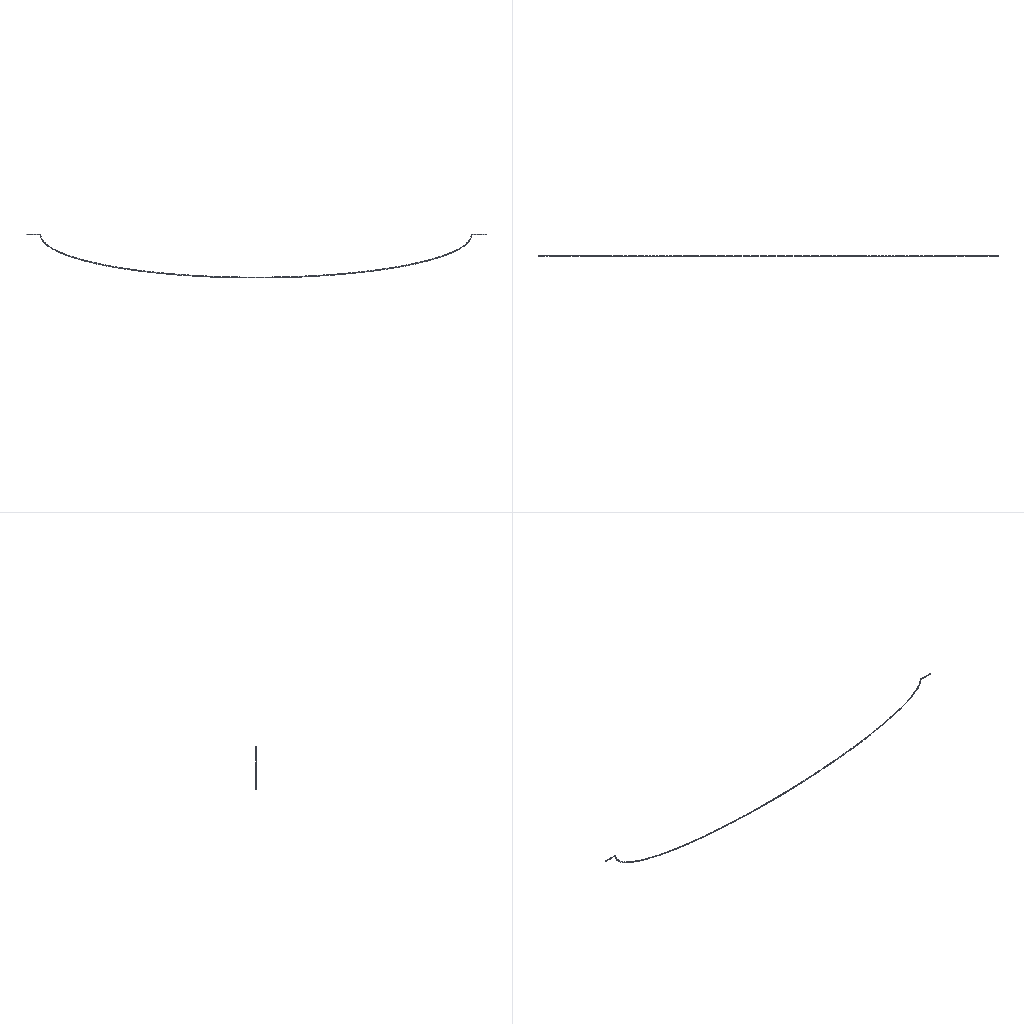Simulation study | ansys workbench
Set-up summary:
category,name,step,type,value,unit,region
solver,ansys_workbench
units,mm-N-s-tonne (MPa),,stated,"/units,MPA"
analysis,LS1,,modal,method=lanb; n_modes=6
load_step,LS1,LS1,modal
mesh,nodes,,,2790
mesh,elements,,,1023
element_type,SOLID187,,,1023
material,Structural Steel,,E,200000,tonne s^-2 mm^-1
material,Structural Steel,,nu,0.3
material,Structural Steel,,density,7.85e-09,tonne mm^-3
material,Structural Steel,,conductivity,60.5,tonne mm s^-3 C^-1
material,Structural Steel,,specific_heat,4.34e+08,mm^2 s^-2 C^-1
material,Structural Steel,,cte,1.2e-05,C^-1
material,Structural Steel,,permeability,10000
material,Structural Steel,,resistivity,0.00017,ohm mm
Ansys APDL input file, long lists of numbers shortened:
/batch
/config,noeldb,1     ! force off writing results to database
*get,_wallstrt,active,,time,wall
! ANSYS input file written by Workbench version 2022 R1
! File used for geometry attach:
/title,wbnew--__ (B5)
! ****** Begin Custom Load Command Snippet ******
/COM, ACT Extensions:
/COM,     LSDYNA, 2021.1
/COM,
! ****** End   Custom Load Command Snippet ******
*DIM,_wb_ProjectScratch_dir,string,248
_wb_ProjectScratch_dir(1) = ''
*DIM,_wb_SolverFiles_dir,string,248
_wb_SolverFiles_dir(1) = ''
*DIM,_wb_userfiles_dir,string,248
_wb_userfiles_dir(1) = ''
/com,--- Data in consistent NMM units. See Solving Units in the help system for more information.
/units,MPA
/nopr
/wb,file,start              !  signify a WB generated input file
/prep7
! Turn off shape checking because checks already performed inside WB mesher.
! See help system for more information.
SHPP,OFF,,NOWARN
/nolist
etcon,set             ! allow ANSYS to choose best KEYOP's for 180x elements, resets any applicable keyopt to MAPDL defaults
/com,*********** Nodes for the whole assembly ***********
nblock,3,,3069
(1i9,3e20.9e3)
        1     1.600000000E+04     0.000000000E+00     3.000000000E+01
! (2789 more lines like these left out)
-1
/wb,elem,start            !  set before creation of elements
/com,*********** Elements for Body 1 "__1-FreeParts|__1" ***********
et,1,187
eblock,19,solid,,1023
(19i9)
        1        1        1        1        0        0        0        0       10        0        1        2      151      589        4      599     1655      600      597
! (2045 more lines like these left out)
-1
/wb,elem,end               !  done creating elements
/com,*********** Send User Defined Coordinate System(s) ***********
csys,0
toffst,273.15,  ! Temperature offset from absolute zero
/com,*********** Set Reference Temperature ***********
tref,22.
/wb,mat,start              !  starting to send materials
/com,*********** Send Materials ***********
Temperature = 'TEMP' ! Temperature
MP,DENS,1,7.85e-09,	! tonne mm^-3
MP,ALPX,1,1.2e-05,	! C^-1
MP,C,1,434000000,	! mm^2 s^-2 C^-1
MP,KXX,1,60.5,	! tonne mm s^-3 C^-1
MP,RSVX,1,0.00017,	! ohm mm
MP,EX,1,200000,	! tonne s^-2 mm^-1
MP,NUXY,1,0.3,
MP,MURX,1,10000,
/wb,mat,end                !  done sending materials
!************************* Model Summary ********************
!__1-FreeParts|__1,	结构钢,	matid,	1
!************************* End Model Summary ********************
! get the diagonal of the bounding box. Needed later for other things
*get,_xmin,node,,mnloc,x
*get,_ymin,node,,mnloc,y
*get,_zmin,node,,mnloc,z
*get,_xmax,node,,mxloc,x
*get,_ymax,node,,mxloc,y
*get,_zmax,node,,mxloc,z
_ASMDIAG=(_xmax-_xmin)*(_xmax-_xmin)+(_ymax-_ymin)*(_ymax-_ymin)+(_zmax-_zmin)*(_zmax-_zmin)
_ASMDIAG=SQRT(_ASMDIAG)
/wb,contact,start          !  starting to send contact
/wb,contact,end            !  done creating contacts
/golist
/wb,load,start             !  starting to send loads
/gst,on,on
fini
*get,_numnode,node,0,count
*get,_numelem,elem,0,count
*get, _MAXELEMNUM, elem, 0, NUM, MAX
*get, _MAXNODENUM, node, 0, NUM, MAX
*get, _MAXELEMTYPE, etyp, 0, NUM, MAX
*get, _MAXREALCONST, real, 0, NUM, MAX
/go
/wb,load,end               !  done creating loads
/com,--- Number of total nodes = %_numnode%
/com,--- Number of contact elements = 0
/com,--- Number of spring elements = 0
/com,--- Number of bearing elements = 0
/com,--- Number of solid elements = 1023
/com,--- Number of condensed parts = 0
/com,--- Number of total elements = %_numelem%
*get,_wallbsol,active,,time,wall
/solu
antype,2                   ! modal analysis
_thickRatio=  0     ! Ratio of thick parts in the model
modopt,lanb,6
outres,erase
outres,all,none
outres,nsol,all
outres,etmp,all
mxpand                    ! default expand in case of complex solution
dmpopt,esav,no
dmpopt,emat,no
dmpopt,full,no
! *********** WB SOLVE COMMAND ***********
! check interactive state
*get,ANSINTER_,active,,int
*if,ANSINTER_,ne,0,then
/eof
*endif
solve
/com *************** Write FE CONNECTORS *********
CEWRITE,file,ce,,INTE
*get,_nmodalsolproc,active,0,numcpu
fini
/nopr
*get,_numnode,node,0,count
*get,_numelem,elem,0,count
*get, _MAXELEMNUM, elem, 0, NUM, MAX
*get, _MAXNODENUM, node, 0, NUM, MAX,,,INTERNAL
*get, _MAXELEMTYPE, etyp, 0, NUM, MAX
*get, _MAXREALCONST, real, 0, NUM, MAX
/gopr
*get,_wallasol,active,,time,wall
/post1
/nopr
*dim,_direction,CHAR,6,1
_direction(1) = 'X'
_direction(2) = 'Y'
_direction(3) = 'Z'
_direction(4) = 'ROTX'
_direction(5) = 'ROTY'
_direction(6) = 'ROTZ'
*get,_lastLS,active,0,set,LSTP
*get,_beginset,active,0,set,nset,first,_lastLS
*get,_endset,active,0,set,nset,last,_lastLS
_nummodes = 0
*if,_endset,gt,0,then
_nummodes = _endset - _beginset + 1
*endif
*do,i_mode,1,_nummodes
   *do,j_component,1,6
			*get,PFACT_%i_mode%_%j_component%,MODE,%i_mode%,PFACT,,DIREC,_direction(%j_component%)
   *enddo
*enddo
*dim,_tmdirection,CHAR,6,1
_tmdirection(1) = 'X'
_tmdirection(2) = 'Y'
_tmdirection(3) = 'Z'
_tmdirection(4) = 'X'
_tmdirection(5) = 'Y'
_tmdirection(6) = 'Z'
*do,j_component,1,6
    *if,j_component,gt,3,then
        *get,TOTALMASS_%j_component%,ELEM,0,IOR,_tmdirection(%j_component%)
    *else
        *get,TOTALMASS_%j_component%,ELEM,0,MTOT,_tmdirection(%j_component%)
    *endif
*enddo
/gopr
xmlo,ENCODING,ISO-8859-1
xmlo,parm
/xml,parm,xml
fini
/gopr
*get,_walldone,active,,time,wall
_preptime=(_wallbsol-_wallstrt)*3600
_solvtime=(_wallasol-_wallbsol)*3600
_posttime=(_walldone-_wallasol)*3600
_totaltim=(_walldone-_wallstrt)*3600
*get,_dlbratio,active,0,solu,dlbr
*get,_combtime,active,0,solu,comb
*get,_ssmode,active,0,solu,ssmm
*get,_ndofs,active,0,solu,ndof
/fclean				!clean distributed files
/com,--- Total number of nodes = %_numnode%
/com,--- Total number of elements = %_numelem%
/com,--- Element load balance ratio = %_dlbratio%
/com,--- Time to combine distributed files = %_combtime%
/com,--- Sparse memory mode = %_ssmode%
/com,--- Number of DOF = %_ndofs%
/wb,file,end               ! done with WB generated input
Results summary:
result,analyses[0].index,,,1
result,analyses[0].system,,,SYS
result,analyses[0].deck,,,deck.dat
result,analyses[0].solve_status,,,completed
result,analyses[0].analysis_type,,,modal
result,analyses[0].physics,,,mechanical
result,analyses[0].unit_system,,,"NMM: mm, ton, N, s, mV, mA, degC"
result,analyses[0].n_sets,,,6
result,analyses[0].modal_frequencies_hz[1],,,0
result,analyses[0].modal_frequencies_hz[2],,,5.44053e-05
result,analyses[0].modal_frequencies_hz[3],,,9.78399e-05
result,analyses[0].modal_frequencies_hz[4],,,0.0001998
result,analyses[0].modal_frequencies_hz[5],,,0.000221
result,analyses[0].modal_frequencies_hz[6],,,0.0003553